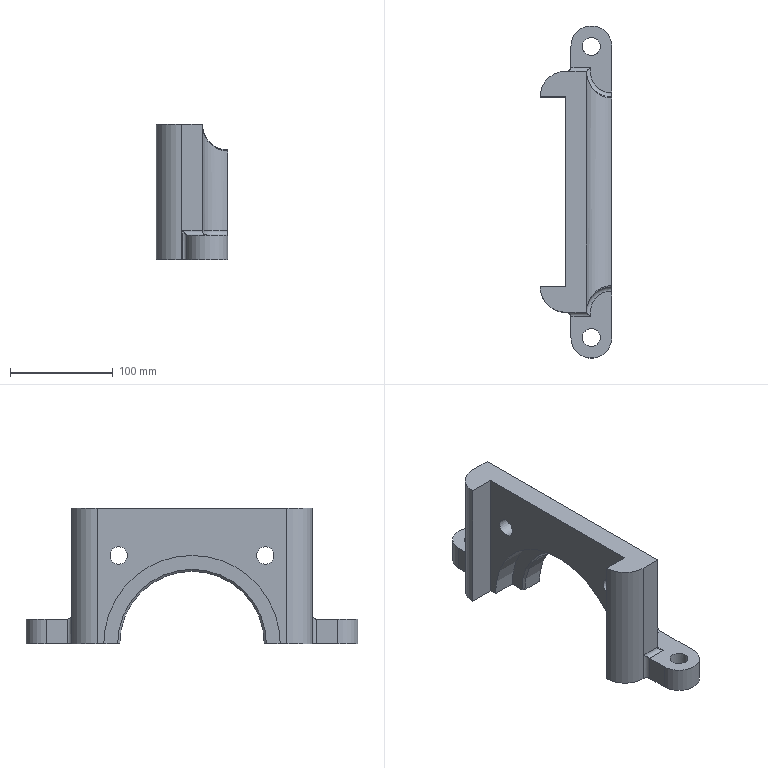Part | NX | features DATUM_CSYS 8, SKETCH 7, EXTRUDE 5, BLEND 4, CBORE_HOLE 2, HOLE PACKAGE 2, SIMPLE HOLE 2, CHAMFER 1, SWP104 1 | 1 solid | 40 faces | box 70 x 324 x 132 mm | volume 928360 mm3 | cylinder 19 | plane 16 | torus 2 | spline 2 | cone 1 | commonest cylinder face diameters 50 x5 8 x4 17 x2 17.5 x2 35 x2 40 x2
STEP:
#1=CARTESIAN_POINT('',(50.,71.5,103.5));
#2=VERTEX_POINT('',#1);
#3=CARTESIAN_POINT('',(50.,71.5,86.));
#4=DIRECTION('',(-1.,0.,0.));
#5=DIRECTION('',(0.,0.,1.));
#6=AXIS2_PLACEMENT_3D('',#3,#4,#5);
#7=CIRCLE('',#6,17.5);
#8=EDGE_CURVE('',#2,#2,#7,.T.);
#9=ORIENTED_EDGE('',*,*,#8,.T.);
#10=EDGE_LOOP('',(#9));
#11=FACE_BOUND('',#10,.T.);
#12=CARTESIAN_POINT('',(50.,-71.5,103.5));
#13=VERTEX_POINT('',#12);
#14=CARTESIAN_POINT('',(50.,-71.5,86.));
#15=DIRECTION('',(-1.,0.,0.));
#16=DIRECTION('',(0.,0.,1.));
#17=AXIS2_PLACEMENT_3D('',#14,#15,#16);
#18=CIRCLE('',#17,17.5);
#19=EDGE_CURVE('',#13,#13,#18,.T.);
#20=ORIENTED_EDGE('',*,*,#19,.T.);
#21=EDGE_LOOP('',(#20));
#22=FACE_BOUND('',#21,.T.);
#23=CARTESIAN_POINT('',(50.,92.5,28.));
#24=VERTEX_POINT('',#23);
#25=CARTESIAN_POINT('',(50.,92.5,106.));
#26=VERTEX_POINT('',#25);
#27=CARTESIAN_POINT('',(50.,92.5,142.8));
#28=DIRECTION('',(0.,0.,-1.));
#29=VECTOR('',#28,1000.);
#30=LINE('',#27,#29);
#31=EDGE_CURVE('',#24,#26,#30,.F.);
#32=ORIENTED_EDGE('',*,*,#31,.T.);
#33=CARTESIAN_POINT('',(50.,91.5,107.));
#34=VERTEX_POINT('',#33);
#35=CARTESIAN_POINT('',(50.,91.5,106.));
#36=DIRECTION('',(1.,0.,0.));
#37=DIRECTION('',(0.,0.,-1.));
#38=AXIS2_PLACEMENT_3D('',#35,#36,#37);
#39=CIRCLE('',#38,1.);
#40=EDGE_CURVE('',#26,#34,#39,.T.);
#41=ORIENTED_EDGE('',*,*,#40,.T.);
#42=CARTESIAN_POINT('',(50.,-91.5,107.));
#43=VERTEX_POINT('',#42);
#44=CARTESIAN_POINT('',(50.,-178.2,107.));
#45=DIRECTION('',(0.,1.,0.));
#46=VECTOR('',#45,1000.);
#47=LINE('',#44,#46);
#48=EDGE_CURVE('',#34,#43,#47,.F.);
#49=ORIENTED_EDGE('',*,*,#48,.T.);
#50=CARTESIAN_POINT('',(50.,-92.5,106.));
#51=VERTEX_POINT('',#50);
#52=CARTESIAN_POINT('',(50.,-91.5,106.));
#53=DIRECTION('',(1.,0.,0.));
#54=DIRECTION('',(0.,0.,-1.));
#55=AXIS2_PLACEMENT_3D('',#52,#53,#54);
#56=CIRCLE('',#55,1.);
#57=EDGE_CURVE('',#43,#51,#56,.T.);
#58=ORIENTED_EDGE('',*,*,#57,.T.);
#59=CARTESIAN_POINT('',(50.,-92.5,28.));
#60=VERTEX_POINT('',#59);
#61=CARTESIAN_POINT('',(50.,-92.5,142.8));
#62=DIRECTION('',(0.,0.,-1.));
#63=VECTOR('',#62,1000.);
#64=LINE('',#61,#63);
#65=EDGE_CURVE('',#60,#51,#64,.F.);
#66=ORIENTED_EDGE('',*,*,#65,.F.);
#67=CARTESIAN_POINT('',(50.,-96.5,24.));
#68=VERTEX_POINT('',#67);
#69=CARTESIAN_POINT('',(50.,-96.5,28.));
#70=DIRECTION('',(1.,0.,0.));
#71=DIRECTION('',(0.,0.,-1.));
#72=AXIS2_PLACEMENT_3D('',#69,#70,#71);
#73=CIRCLE('',#72,4.);
#74=EDGE_CURVE('',#60,#68,#73,.F.);
#75=ORIENTED_EDGE('',*,*,#74,.T.);
#76=CARTESIAN_POINT('',(50.,-142.,24.));
#77=VERTEX_POINT('',#76);
#78=CARTESIAN_POINT('',(50.,-117.5,24.));
#79=DIRECTION('',(0.,-1.,0.));
#80=VECTOR('',#79,1000.);
#81=LINE('',#78,#80);
#82=EDGE_CURVE('',#68,#77,#81,.T.);
#83=ORIENTED_EDGE('',*,*,#82,.T.);
#84=CARTESIAN_POINT('',(50.,-142.,0.));
#85=VERTEX_POINT('',#84);
#86=CARTESIAN_POINT('',(50.,-142.,0.));
#87=DIRECTION('',(0.,0.,-1.));
#88=VECTOR('',#87,1000.);
#89=LINE('',#86,#88);
#90=EDGE_CURVE('',#77,#85,#89,.T.);
#91=ORIENTED_EDGE('',*,*,#90,.T.);
#92=CARTESIAN_POINT('',(50.,-70.5,0.));
#93=VERTEX_POINT('',#92);
#94=CARTESIAN_POINT('',(50.,-162.,0.));
#95=DIRECTION('',(0.,1.,0.));
#96=VECTOR('',#95,1000.);
#97=LINE('',#94,#96);
#98=EDGE_CURVE('',#85,#93,#97,.T.);
#99=ORIENTED_EDGE('',*,*,#98,.T.);
#100=CARTESIAN_POINT('',(50.,70.5,0.));
#101=VERTEX_POINT('',#100);
#102=CARTESIAN_POINT('',(50.,0.,0.));
#103=DIRECTION('',(1.,0.,0.));
#104=DIRECTION('',(0.,0.,-1.));
#105=AXIS2_PLACEMENT_3D('',#102,#103,#104);
#106=CIRCLE('',#105,70.5);
#107=EDGE_CURVE('',#101,#93,#106,.T.);
#108=ORIENTED_EDGE('',*,*,#107,.F.);
#109=CARTESIAN_POINT('',(50.,142.,0.));
#110=VERTEX_POINT('',#109);
#111=CARTESIAN_POINT('',(50.,-162.,0.));
#112=DIRECTION('',(0.,1.,0.));
#113=VECTOR('',#112,1000.);
#114=LINE('',#111,#113);
#115=EDGE_CURVE('',#101,#110,#114,.T.);
#116=ORIENTED_EDGE('',*,*,#115,.T.);
#117=CARTESIAN_POINT('',(50.,142.,24.));
#118=VERTEX_POINT('',#117);
#119=CARTESIAN_POINT('',(50.,142.,24.));
#120=DIRECTION('',(0.,0.,1.));
#121=VECTOR('',#120,1000.);
#122=LINE('',#119,#121);
#123=EDGE_CURVE('',#110,#118,#122,.T.);
#124=ORIENTED_EDGE('',*,*,#123,.T.);
#125=CARTESIAN_POINT('',(50.,96.5,24.));
#126=VERTEX_POINT('',#125);
#127=CARTESIAN_POINT('',(50.,162.,24.));
#128=DIRECTION('',(0.,-1.,0.));
#129=VECTOR('',#128,1000.);
#130=LINE('',#127,#129);
#131=EDGE_CURVE('',#118,#126,#130,.T.);
#132=ORIENTED_EDGE('',*,*,#131,.T.);
#133=CARTESIAN_POINT('',(50.,96.5,28.));
#134=DIRECTION('',(1.,0.,0.));
#135=DIRECTION('',(0.,0.,-1.));
#136=AXIS2_PLACEMENT_3D('',#133,#134,#135);
#137=CIRCLE('',#136,4.);
#138=EDGE_CURVE('',#126,#24,#137,.F.);
#139=ORIENTED_EDGE('',*,*,#138,.T.);
#140=EDGE_LOOP('',(#32,#41,#49,#58,#66,#75,#83,#91,#99,#108,#116,#124,#132,#139));
#141=FACE_BOUND('',#140,.T.);
#142=CARTESIAN_POINT('',(50.,0.,0.));
#143=DIRECTION('',(1.,0.,0.));
#144=DIRECTION('',(0.,0.,-1.));
#145=AXIS2_PLACEMENT_3D('',#142,#143,#144);
#146=PLANE('',#145);
#147=ADVANCED_FACE('',(#11,#22,#141),#146,.T.);
#148=CARTESIAN_POINT('',(25.,117.5,28.));
#149=VERTEX_POINT('',#148);
#150=CARTESIAN_POINT('',(6.,117.5,28.));
#151=VERTEX_POINT('',#150);
#152=CARTESIAN_POINT('',(10.,117.5,28.));
#153=DIRECTION('',(-1.,0.,0.));
#154=VECTOR('',#153,1000.);
#155=LINE('',#152,#154);
#156=EDGE_CURVE('',#149,#151,#155,.T.);
#157=ORIENTED_EDGE('',*,*,#156,.T.);
#158=CARTESIAN_POINT('',(6.,117.5,0.));
#159=VERTEX_POINT('',#158);
#160=CARTESIAN_POINT('',(6.,117.5,0.));
#161=DIRECTION('',(0.,0.,-1.));
#162=VECTOR('',#161,1000.);
#163=LINE('',#160,#162);
#164=EDGE_CURVE('',#151,#159,#163,.T.);
#165=ORIENTED_EDGE('',*,*,#164,.T.);
#166=CARTESIAN_POINT('',(5.,117.5,0.));
#167=VERTEX_POINT('',#166);
#168=CARTESIAN_POINT('',(10.,117.5,0.));
#169=DIRECTION('',(-1.,0.,0.));
#170=VECTOR('',#169,1000.);
#171=LINE('',#168,#170);
#172=EDGE_CURVE('',#167,#159,#171,.F.);
#173=ORIENTED_EDGE('',*,*,#172,.F.);
#174=CARTESIAN_POINT('',(5.,117.5,132.));
#175=VERTEX_POINT('',#174);
#176=CARTESIAN_POINT('',(5.,117.5,24.));
#177=DIRECTION('',(0.,0.,1.));
#178=VECTOR('',#177,1000.);
#179=LINE('',#176,#178);
#180=EDGE_CURVE('',#167,#175,#179,.T.);
#181=ORIENTED_EDGE('',*,*,#180,.T.);
#182=CARTESIAN_POINT('',(25.,117.5,132.));
#183=VERTEX_POINT('',#182);
#184=CARTESIAN_POINT('',(50.,117.5,132.));
#185=DIRECTION('',(-1.,0.,0.));
#186=VECTOR('',#185,1000.);
#187=LINE('',#184,#186);
#188=EDGE_CURVE('',#183,#175,#187,.T.);
#189=ORIENTED_EDGE('',*,*,#188,.F.);
#190=CARTESIAN_POINT('',(25.,117.5,142.8));
#191=DIRECTION('',(0.,0.,-1.));
#192=VECTOR('',#191,1000.);
#193=LINE('',#190,#192);
#194=EDGE_CURVE('',#149,#183,#193,.F.);
#195=ORIENTED_EDGE('',*,*,#194,.F.);
#196=EDGE_LOOP('',(#157,#165,#173,#181,#189,#195));
#197=FACE_BOUND('',#196,.T.);
#198=CARTESIAN_POINT('',(50.,117.5,24.));
#199=DIRECTION('',(0.,-1.,0.));
#200=DIRECTION('',(0.,0.,-1.));
#201=AXIS2_PLACEMENT_3D('',#198,#199,#200);
#202=PLANE('',#201);
#203=ADVANCED_FACE('',(#197),#202,.F.);
#204=ORIENTED_EDGE('',*,*,#48,.F.);
#205=CARTESIAN_POINT('',(50.,117.5,132.));
#206=DIRECTION('',(0.,-0.6931,0.7208));
#207=DIRECTION('',(0.,0.7208,0.6931));
#208=AXIS2_PLACEMENT_3D('',#205,#206,#207);
#209=ELLIPSE('',#208,36.069,25.);
#210=EDGE_CURVE('',#34,#183,#209,.F.);
#211=ORIENTED_EDGE('',*,*,#210,.T.);
#212=CARTESIAN_POINT('',(25.,-117.5,132.));
#213=VERTEX_POINT('',#212);
#214=CARTESIAN_POINT('',(25.,-178.2,132.));
#215=DIRECTION('',(0.,1.,0.));
#216=VECTOR('',#215,1000.);
#217=LINE('',#214,#216);
#218=EDGE_CURVE('',#183,#213,#217,.F.);
#219=ORIENTED_EDGE('',*,*,#218,.T.);
#220=CARTESIAN_POINT('',(50.,-117.5,132.));
#221=DIRECTION('',(0.,0.6931,0.7208));
#222=DIRECTION('',(0.,0.7208,-0.6931));
#223=AXIS2_PLACEMENT_3D('',#220,#221,#222);
#224=ELLIPSE('',#223,36.069,25.);
#225=EDGE_CURVE('',#213,#43,#224,.F.);
#226=ORIENTED_EDGE('',*,*,#225,.T.);
#227=EDGE_LOOP('',(#204,#211,#219,#226));
#228=FACE_BOUND('',#227,.T.);
#229=CARTESIAN_POINT('',(50.,-178.2,132.));
#230=DIRECTION('',(0.,1.,0.));
#231=DIRECTION('',(0.,0.,1.));
#232=AXIS2_PLACEMENT_3D('',#229,#230,#231);
#233=CYLINDRICAL_SURFACE('',#232,25.);
#234=ADVANCED_FACE('',(#228),#233,.F.);
#235=CARTESIAN_POINT('',(38.75,142.,0.));
#236=VERTEX_POINT('',#235);
#237=CARTESIAN_POINT('',(30.,142.,0.));
#238=DIRECTION('',(0.,0.,1.));
#239=DIRECTION('',(1.,0.,0.));
#240=AXIS2_PLACEMENT_3D('',#237,#238,#239);
#241=CIRCLE('',#240,8.75);
#242=EDGE_CURVE('',#236,#236,#241,.T.);
#243=ORIENTED_EDGE('',*,*,#242,.T.);
#244=EDGE_LOOP('',(#243));
#245=FACE_BOUND('',#244,.T.);
#246=CARTESIAN_POINT('',(30.,70.5,0.));
#247=VERTEX_POINT('',#246);
#248=CARTESIAN_POINT('',(50.,70.5,0.));
#249=DIRECTION('',(1.,0.,0.));
#250=VECTOR('',#249,1000.);
#251=LINE('',#248,#250);
#252=EDGE_CURVE('',#101,#247,#251,.F.);
#253=ORIENTED_EDGE('',*,*,#252,.T.);
#254=CARTESIAN_POINT('',(28.,72.5,0.));
#255=VERTEX_POINT('',#254);
#256=CARTESIAN_POINT('',(100.5,0.,0.));
#257=DIRECTION('',(-0.7071,0.7071,0.));
#258=VECTOR('',#257,1000.);
#259=LINE('',#256,#258);
#260=EDGE_CURVE('',#247,#255,#259,.T.);
#261=ORIENTED_EDGE('',*,*,#260,.T.);
#262=CARTESIAN_POINT('',(28.,86.,0.));
#263=VERTEX_POINT('',#262);
#264=CARTESIAN_POINT('',(28.,-162.,0.));
#265=DIRECTION('',(0.,1.,0.));
#266=VECTOR('',#265,1000.);
#267=LINE('',#264,#266);
#268=EDGE_CURVE('',#255,#263,#267,.T.);
#269=ORIENTED_EDGE('',*,*,#268,.T.);
#270=CARTESIAN_POINT('',(5.,86.,0.));
#271=VERTEX_POINT('',#270);
#272=CARTESIAN_POINT('',(50.,86.,0.));
#273=DIRECTION('',(1.,0.,0.));
#274=VECTOR('',#273,1000.);
#275=LINE('',#272,#274);
#276=EDGE_CURVE('',#263,#271,#275,.F.);
#277=ORIENTED_EDGE('',*,*,#276,.T.);
#278=CARTESIAN_POINT('',(5.,92.5,0.));
#279=VERTEX_POINT('',#278);
#280=CARTESIAN_POINT('',(5.,92.5,0.));
#281=DIRECTION('',(0.,-1.,0.));
#282=VECTOR('',#281,1000.);
#283=LINE('',#280,#282);
#284=EDGE_CURVE('',#279,#271,#283,.T.);
#285=ORIENTED_EDGE('',*,*,#284,.F.);
#286=CARTESIAN_POINT('',(-20.,92.5,0.));
#287=VERTEX_POINT('',#286);
#288=CARTESIAN_POINT('',(-20.,92.5,0.));
#289=DIRECTION('',(1.,0.,0.));
#290=VECTOR('',#289,1000.);
#291=LINE('',#288,#290);
#292=EDGE_CURVE('',#287,#279,#291,.T.);
#293=ORIENTED_EDGE('',*,*,#292,.F.);
#294=CARTESIAN_POINT('',(5.,92.5,0.));
#295=DIRECTION('',(0.,0.,1.));
#296=DIRECTION('',(1.,0.,0.));
#297=AXIS2_PLACEMENT_3D('',#294,#295,#296);
#298=CIRCLE('',#297,25.);
#299=EDGE_CURVE('',#287,#167,#298,.F.);
#300=ORIENTED_EDGE('',*,*,#299,.T.);
#301=ORIENTED_EDGE('',*,*,#172,.T.);
#302=CARTESIAN_POINT('',(10.,121.5,0.));
#303=VERTEX_POINT('',#302);
#304=CARTESIAN_POINT('',(6.,121.5,0.));
#305=DIRECTION('',(0.,0.,1.));
#306=DIRECTION('',(1.,0.,0.));
#307=AXIS2_PLACEMENT_3D('',#304,#305,#306);
#308=CIRCLE('',#307,4.);
#309=EDGE_CURVE('',#159,#303,#308,.T.);
#310=ORIENTED_EDGE('',*,*,#309,.T.);
#311=CARTESIAN_POINT('',(10.,142.,0.));
#312=VERTEX_POINT('',#311);
#313=CARTESIAN_POINT('',(10.,162.,0.));
#314=DIRECTION('',(0.,-1.,0.));
#315=VECTOR('',#314,1000.);
#316=LINE('',#313,#315);
#317=EDGE_CURVE('',#312,#303,#316,.T.);
#318=ORIENTED_EDGE('',*,*,#317,.F.);
#319=CARTESIAN_POINT('',(30.,142.,0.));
#320=DIRECTION('',(0.,0.,1.));
#321=DIRECTION('',(1.,0.,0.));
#322=AXIS2_PLACEMENT_3D('',#319,#320,#321);
#323=CIRCLE('',#322,20.);
#324=EDGE_CURVE('',#312,#110,#323,.F.);
#325=ORIENTED_EDGE('',*,*,#324,.T.);
#326=ORIENTED_EDGE('',*,*,#115,.F.);
#327=EDGE_LOOP('',(#253,#261,#269,#277,#285,#293,#300,#301,#310,#318,#325,#326));
#328=FACE_BOUND('',#327,.T.);
#329=CARTESIAN_POINT('',(50.,-162.,0.));
#330=DIRECTION('',(0.,0.,1.));
#331=DIRECTION('',(1.,0.,0.));
#332=AXIS2_PLACEMENT_3D('',#329,#330,#331);
#333=PLANE('',#332);
#334=ADVANCED_FACE('',(#245,#328),#333,.F.);
#335=CARTESIAN_POINT('',(38.75,-142.,0.));
#336=VERTEX_POINT('',#335);
#337=CARTESIAN_POINT('',(30.,-142.,0.));
#338=DIRECTION('',(0.,0.,1.));
#339=DIRECTION('',(1.,0.,0.));
#340=AXIS2_PLACEMENT_3D('',#337,#338,#339);
#341=CIRCLE('',#340,8.75);
#342=EDGE_CURVE('',#336,#336,#341,.T.);
#343=ORIENTED_EDGE('',*,*,#342,.T.);
#344=EDGE_LOOP('',(#343));
#345=FACE_BOUND('',#344,.T.);
#346=CARTESIAN_POINT('',(28.,-86.,0.));
#347=VERTEX_POINT('',#346);
#348=CARTESIAN_POINT('',(28.,-72.5,0.));
#349=VERTEX_POINT('',#348);
#350=CARTESIAN_POINT('',(28.,-162.,0.));
#351=DIRECTION('',(0.,1.,0.));
#352=VECTOR('',#351,1000.);
#353=LINE('',#350,#352);
#354=EDGE_CURVE('',#347,#349,#353,.T.);
#355=ORIENTED_EDGE('',*,*,#354,.T.);
#356=CARTESIAN_POINT('',(30.,-70.5,0.));
#357=VERTEX_POINT('',#356);
#358=CARTESIAN_POINT('',(100.5,0.,0.));
#359=DIRECTION('',(0.7071,0.7071,0.));
#360=VECTOR('',#359,1000.);
#361=LINE('',#358,#360);
#362=EDGE_CURVE('',#349,#357,#361,.T.);
#363=ORIENTED_EDGE('',*,*,#362,.T.);
#364=CARTESIAN_POINT('',(50.,-70.5,0.));
#365=DIRECTION('',(1.,0.,0.));
#366=VECTOR('',#365,1000.);
#367=LINE('',#364,#366);
#368=EDGE_CURVE('',#357,#93,#367,.T.);
#369=ORIENTED_EDGE('',*,*,#368,.T.);
#370=ORIENTED_EDGE('',*,*,#98,.F.);
#371=CARTESIAN_POINT('',(10.,-142.,0.));
#372=VERTEX_POINT('',#371);
#373=CARTESIAN_POINT('',(30.,-142.,0.));
#374=DIRECTION('',(0.,0.,1.));
#375=DIRECTION('',(1.,0.,0.));
#376=AXIS2_PLACEMENT_3D('',#373,#374,#375);
#377=CIRCLE('',#376,20.);
#378=EDGE_CURVE('',#85,#372,#377,.F.);
#379=ORIENTED_EDGE('',*,*,#378,.T.);
#380=CARTESIAN_POINT('',(10.,-121.5,0.));
#381=VERTEX_POINT('',#380);
#382=CARTESIAN_POINT('',(10.,-162.,0.));
#383=DIRECTION('',(0.,1.,0.));
#384=VECTOR('',#383,1000.);
#385=LINE('',#382,#384);
#386=EDGE_CURVE('',#372,#381,#385,.T.);
#387=ORIENTED_EDGE('',*,*,#386,.T.);
#388=CARTESIAN_POINT('',(6.,-117.5,0.));
#389=VERTEX_POINT('',#388);
#390=CARTESIAN_POINT('',(6.,-121.5,0.));
#391=DIRECTION('',(0.,0.,1.));
#392=DIRECTION('',(1.,0.,0.));
#393=AXIS2_PLACEMENT_3D('',#390,#391,#392);
#394=CIRCLE('',#393,4.);
#395=EDGE_CURVE('',#381,#389,#394,.T.);
#396=ORIENTED_EDGE('',*,*,#395,.T.);
#397=CARTESIAN_POINT('',(5.,-117.5,0.));
#398=VERTEX_POINT('',#397);
#399=CARTESIAN_POINT('',(10.,-117.5,0.));
#400=DIRECTION('',(-1.,0.,0.));
#401=VECTOR('',#400,1000.);
#402=LINE('',#399,#401);
#403=EDGE_CURVE('',#389,#398,#402,.T.);
#404=ORIENTED_EDGE('',*,*,#403,.T.);
#405=CARTESIAN_POINT('',(-20.,-92.5,0.));
#406=VERTEX_POINT('',#405);
#407=CARTESIAN_POINT('',(5.,-92.5,0.));
#408=DIRECTION('',(0.,0.,1.));
#409=DIRECTION('',(1.,0.,0.));
#410=AXIS2_PLACEMENT_3D('',#407,#408,#409);
#411=CIRCLE('',#410,25.);
#412=EDGE_CURVE('',#398,#406,#411,.F.);
#413=ORIENTED_EDGE('',*,*,#412,.T.);
#414=CARTESIAN_POINT('',(5.,-92.5,0.));
#415=VERTEX_POINT('',#414);
#416=CARTESIAN_POINT('',(5.,-92.5,0.));
#417=DIRECTION('',(-1.,0.,0.));
#418=VECTOR('',#417,1000.);
#419=LINE('',#416,#418);
#420=EDGE_CURVE('',#415,#406,#419,.T.);
#421=ORIENTED_EDGE('',*,*,#420,.F.);
#422=CARTESIAN_POINT('',(5.,-86.,0.));
#423=VERTEX_POINT('',#422);
#424=CARTESIAN_POINT('',(5.,92.5,0.));
#425=DIRECTION('',(0.,-1.,0.));
#426=VECTOR('',#425,1000.);
#427=LINE('',#424,#426);
#428=EDGE_CURVE('',#423,#415,#427,.T.);
#429=ORIENTED_EDGE('',*,*,#428,.F.);
#430=CARTESIAN_POINT('',(50.,-86.,0.));
#431=DIRECTION('',(1.,0.,0.));
#432=VECTOR('',#431,1000.);
#433=LINE('',#430,#432);
#434=EDGE_CURVE('',#423,#347,#433,.T.);
#435=ORIENTED_EDGE('',*,*,#434,.T.);
#436=EDGE_LOOP('',(#355,#363,#369,#370,#379,#387,#396,#404,#413,#421,#429,#435));
#437=FACE_BOUND('',#436,.T.);
#438=CARTESIAN_POINT('',(50.,-162.,0.));
#439=DIRECTION('',(0.,0.,1.));
#440=DIRECTION('',(1.,0.,0.));
#441=AXIS2_PLACEMENT_3D('',#438,#439,#440);
#442=PLANE('',#441);
#443=ADVANCED_FACE('',(#345,#437),#442,.F.);
#444=CARTESIAN_POINT('',(5.,-92.5,132.));
#445=VERTEX_POINT('',#444);
#446=CARTESIAN_POINT('',(-20.,-92.5,132.));
#447=VERTEX_POINT('',#446);
#448=CARTESIAN_POINT('',(50.,-92.5,132.));
#449=DIRECTION('',(-1.,0.,0.));
#450=VECTOR('',#449,1000.);
#451=LINE('',#448,#450);
#452=EDGE_CURVE('',#445,#447,#451,.T.);
#453=ORIENTED_EDGE('',*,*,#452,.T.);
#454=CARTESIAN_POINT('',(5.,-117.5,132.));
#455=VERTEX_POINT('',#454);
#456=CARTESIAN_POINT('',(5.,-92.5,132.));
#457=DIRECTION('',(0.,0.,-1.));
#458=DIRECTION('',(0.,1.,0.));
#459=AXIS2_PLACEMENT_3D('',#456,#457,#458);
#460=CIRCLE('',#459,25.);
#461=EDGE_CURVE('',#447,#455,#460,.F.);
#462=ORIENTED_EDGE('',*,*,#461,.T.);
#463=CARTESIAN_POINT('',(50.,-117.5,132.));
#464=DIRECTION('',(-1.,0.,0.));
#465=VECTOR('',#464,1000.);
#466=LINE('',#463,#465);
#467=EDGE_CURVE('',#213,#455,#466,.T.);
#468=ORIENTED_EDGE('',*,*,#467,.F.);
#469=ORIENTED_EDGE('',*,*,#218,.F.);
#470=ORIENTED_EDGE('',*,*,#188,.T.);
#471=CARTESIAN_POINT('',(-20.,92.5,132.));
#472=VERTEX_POINT('',#471);
#473=CARTESIAN_POINT('',(5.,92.5,132.));
#474=DIRECTION('',(0.,0.,-1.));
#475=DIRECTION('',(0.,1.,0.));
#476=AXIS2_PLACEMENT_3D('',#473,#474,#475);
#477=CIRCLE('',#476,25.);
#478=EDGE_CURVE('',#175,#472,#477,.F.);
#479=ORIENTED_EDGE('',*,*,#478,.T.);
#480=CARTESIAN_POINT('',(5.,92.5,132.));
#481=VERTEX_POINT('',#480);
#482=CARTESIAN_POINT('',(50.,92.5,132.));
#483=DIRECTION('',(1.,0.,0.));
#484=VECTOR('',#483,1000.);
#485=LINE('',#482,#484);
#486=EDGE_CURVE('',#472,#481,#485,.T.);
#487=ORIENTED_EDGE('',*,*,#486,.T.);
#488=CARTESIAN_POINT('',(5.,117.5,132.));
#489=DIRECTION('',(0.,-1.,0.));
#490=VECTOR('',#489,1000.);
#491=LINE('',#488,#490);
#492=EDGE_CURVE('',#481,#445,#491,.T.);
#493=ORIENTED_EDGE('',*,*,#492,.T.);
#494=EDGE_LOOP('',(#453,#462,#468,#469,#470,#479,#487,#493));
#495=FACE_BOUND('',#494,.T.);
#496=CARTESIAN_POINT('',(50.,117.5,132.));
#497=DIRECTION('',(0.,0.,-1.));
#498=DIRECTION('',(0.,1.,0.));
#499=AXIS2_PLACEMENT_3D('',#496,#497,#498);
#500=PLANE('',#499);
#501=ADVANCED_FACE('',(#495),#500,.F.);
#502=CARTESIAN_POINT('',(30.,150.75,24.));
#503=VERTEX_POINT('',#502);
#504=CARTESIAN_POINT('',(30.,142.,24.));
#505=DIRECTION('',(0.,0.,-1.));
#506=DIRECTION('',(0.,1.,0.));
#507=AXIS2_PLACEMENT_3D('',#504,#505,#506);
#508=CIRCLE('',#507,8.75);
#509=EDGE_CURVE('',#503,#503,#508,.T.);
#510=ORIENTED_EDGE('',*,*,#509,.T.);
#511=EDGE_LOOP('',(#510));
#512=FACE_BOUND('',#511,.T.);
#513=CARTESIAN_POINT('',(10.,121.5,24.));
#514=VERTEX_POINT('',#513);
#515=CARTESIAN_POINT('',(10.,142.,24.));
#516=VERTEX_POINT('',#515);
#517=CARTESIAN_POINT('',(10.,162.,24.));
#518=DIRECTION('',(0.,1.,0.));
#519=VECTOR('',#518,1000.);
#520=LINE('',#517,#519);
#521=EDGE_CURVE('',#514,#516,#520,.T.);
#522=ORIENTED_EDGE('',*,*,#521,.F.);
#523=CARTESIAN_POINT('',(29.384,121.5,24.));
#524=VERTEX_POINT('',#523);
#525=CARTESIAN_POINT('',(25.,121.5,24.));
#526=DIRECTION('',(-1.,0.,0.));
#527=VECTOR('',#526,1000.);
#528=LINE('',#525,#527);
#529=EDGE_CURVE('',#514,#524,#528,.F.);
#530=ORIENTED_EDGE('',*,*,#529,.T.);
#531=CARTESIAN_POINT('',(50.,117.5,24.));
#532=DIRECTION('',(0.,0.,-1.));
#533=DIRECTION('',(0.,1.,0.));
#534=AXIS2_PLACEMENT_3D('',#531,#532,#533);
#535=CIRCLE('',#534,21.);
#536=EDGE_CURVE('',#524,#126,#535,.F.);
#537=ORIENTED_EDGE('',*,*,#536,.T.);
#538=ORIENTED_EDGE('',*,*,#131,.F.);
#539=CARTESIAN_POINT('',(30.,142.,24.));
#540=DIRECTION('',(0.,0.,-1.));
#541=DIRECTION('',(0.,1.,0.));
#542=AXIS2_PLACEMENT_3D('',#539,#540,#541);
#543=CIRCLE('',#542,20.);
#544=EDGE_CURVE('',#118,#516,#543,.F.);
#545=ORIENTED_EDGE('',*,*,#544,.T.);
#546=EDGE_LOOP('',(#522,#530,#537,#538,#545));
#547=FACE_BOUND('',#546,.T.);
#548=CARTESIAN_POINT('',(50.,162.,24.));
#549=DIRECTION('',(0.,0.,-1.));
#550=DIRECTION('',(0.,1.,0.));
#551=AXIS2_PLACEMENT_3D('',#548,#549,#550);
#552=PLANE('',#551);
#553=ADVANCED_FACE('',(#512,#547),#552,.F.);
#554=ORIENTED_EDGE('',*,*,#403,.F.);
#555=CARTESIAN_POINT('',(6.,-117.5,28.));
#556=VERTEX_POINT('',#555);
#557=CARTESIAN_POINT('',(6.,-117.5,132.));
#558=DIRECTION('',(0.,0.,-1.));
#559=VECTOR('',#558,1000.);
#560=LINE('',#557,#559);
#561=EDGE_CURVE('',#389,#556,#560,.F.);
#562=ORIENTED_EDGE('',*,*,#561,.T.);
#563=CARTESIAN_POINT('',(25.,-117.5,28.));
#564=VERTEX_POINT('',#563);
#565=CARTESIAN_POINT('',(25.,-117.5,28.));
#566=DIRECTION('',(-1.,0.,0.));
#567=VECTOR('',#566,1000.);
#568=LINE('',#565,#567);
#569=EDGE_CURVE('',#556,#564,#568,.F.);
#570=ORIENTED_EDGE('',*,*,#569,.T.);
#571=CARTESIAN_POINT('',(25.,-117.5,142.8));
#572=DIRECTION('',(0.,0.,-1.));
#573=VECTOR('',#572,1000.);
#574=LINE('',#571,#573);
#575=EDGE_CURVE('',#564,#213,#574,.F.);
#576=ORIENTED_EDGE('',*,*,#575,.T.);
#577=ORIENTED_EDGE('',*,*,#467,.T.);
#578=CARTESIAN_POINT('',(5.,-117.5,132.));
#579=DIRECTION('',(0.,0.,-1.));
#580=VECTOR('',#579,1000.);
#581=LINE('',#578,#580);
#582=EDGE_CURVE('',#455,#398,#581,.T.);
#583=ORIENTED_EDGE('',*,*,#582,.T.);
#584=EDGE_LOOP('',(#554,#562,#570,#576,#577,#583));
#585=FACE_BOUND('',#584,.T.);
#586=CARTESIAN_POINT('',(50.,-117.5,132.));
#587=DIRECTION('',(0.,1.,0.));
#588=DIRECTION('',(0.,0.,1.));
#589=AXIS2_PLACEMENT_3D('',#586,#587,#588);
#590=PLANE('',#589);
#591=ADVANCED_FACE('',(#585),#590,.F.);
#592=CARTESIAN_POINT('',(30.,-133.25,24.));
#593=VERTEX_POINT('',#592);
#594=CARTESIAN_POINT('',(30.,-142.,24.));
#595=DIRECTION('',(0.,0.,-1.));
#596=DIRECTION('',(0.,1.,0.));
#597=AXIS2_PLACEMENT_3D('',#594,#595,#596);
#598=CIRCLE('',#597,8.75);
#599=EDGE_CURVE('',#593,#593,#598,.T.);
#600=ORIENTED_EDGE('',*,*,#599,.T.);
#601=EDGE_LOOP('',(#600));
#602=FACE_BOUND('',#601,.T.);
#603=CARTESIAN_POINT('',(29.384,-121.5,24.));
#604=VERTEX_POINT('',#603);
#605=CARTESIAN_POINT('',(50.,-117.5,24.));
#606=DIRECTION('',(0.,0.,-1.));
#607=DIRECTION('',(0.,1.,0.));
#608=AXIS2_PLACEMENT_3D('',#605,#606,#607);
#609=CIRCLE('',#608,21.);
#610=EDGE_CURVE('',#68,#604,#609,.F.);
#611=ORIENTED_EDGE('',*,*,#610,.T.);
#612=CARTESIAN_POINT('',(10.,-121.5,24.));
#613=VERTEX_POINT('',#612);
#614=CARTESIAN_POINT('',(10.,-121.5,24.));
#615=DIRECTION('',(-1.,0.,0.));
#616=VECTOR('',#615,1000.);
#617=LINE('',#614,#616);
#618=EDGE_CURVE('',#604,#613,#617,.T.);
#619=ORIENTED_EDGE('',*,*,#618,.T.);
#620=CARTESIAN_POINT('',(10.,-142.,24.));
#621=VERTEX_POINT('',#620);
#622=CARTESIAN_POINT('',(10.,-162.,24.));
#623=DIRECTION('',(0.,-1.,0.));
#624=VECTOR('',#623,1000.);
#625=LINE('',#622,#624);
#626=EDGE_CURVE('',#613,#621,#625,.T.);
#627=ORIENTED_EDGE('',*,*,#626,.T.);
#628=CARTESIAN_POINT('',(30.,-142.,24.));
#629=DIRECTION('',(0.,0.,-1.));
#630=DIRECTION('',(0.,1.,0.));
#631=AXIS2_PLACEMENT_3D('',#628,#629,#630);
#632=CIRCLE('',#631,20.);
#633=EDGE_CURVE('',#621,#77,#632,.F.);
#634=ORIENTED_EDGE('',*,*,#633,.T.);
#635=ORIENTED_EDGE('',*,*,#82,.F.);
#636=EDGE_LOOP('',(#611,#619,#627,#634,#635));
#637=FACE_BOUND('',#636,.T.);
#638=CARTESIAN_POINT('',(50.,-117.5,24.));
#639=DIRECTION('',(0.,0.,-1.));
#640=DIRECTION('',(0.,1.,0.));
#641=AXIS2_PLACEMENT_3D('',#638,#639,#640);
#642=PLANE('',#641);
#643=ADVANCED_FACE('',(#602,#637),#642,.F.);
#644=ORIENTED_EDGE('',*,*,#626,.F.);
#645=CARTESIAN_POINT('',(10.,-121.5,145.2));
#646=DIRECTION('',(0.,0.,-1.));
#647=VECTOR('',#646,1000.);
#648=LINE('',#645,#647);
#649=EDGE_CURVE('',#613,#381,#648,.T.);
#650=ORIENTED_EDGE('',*,*,#649,.T.);
#651=ORIENTED_EDGE('',*,*,#386,.F.);
#652=CARTESIAN_POINT('',(10.,-142.,24.));
#653=DIRECTION('',(0.,0.,-1.));
#654=VECTOR('',#653,1000.);
#655=LINE('',#652,#654);
#656=EDGE_CURVE('',#372,#621,#655,.F.);
#657=ORIENTED_EDGE('',*,*,#656,.T.);
#658=EDGE_LOOP('',(#644,#650,#651,#657));
#659=FACE_BOUND('',#658,.T.);
#660=CARTESIAN_POINT('',(10.,-162.,145.2));
#661=DIRECTION('',(-1.,0.,0.));
#662=DIRECTION('',(0.,-1.,0.));
#663=AXIS2_PLACEMENT_3D('',#660,#661,#662);
#664=PLANE('',#663);
#665=ADVANCED_FACE('',(#659),#664,.T.);
#666=ORIENTED_EDGE('',*,*,#317,.T.);
#667=CARTESIAN_POINT('',(10.,121.5,24.));
#668=DIRECTION('',(0.,0.,-1.));
#669=VECTOR('',#668,1000.);
#670=LINE('',#667,#669);
#671=EDGE_CURVE('',#303,#514,#670,.F.);
#672=ORIENTED_EDGE('',*,*,#671,.T.);
#673=ORIENTED_EDGE('',*,*,#521,.T.);
#674=CARTESIAN_POINT('',(10.,142.,145.2));
#675=DIRECTION('',(0.,0.,-1.));
#676=VECTOR('',#675,1000.);
#677=LINE('',#674,#676);
#678=EDGE_CURVE('',#516,#312,#677,.T.);
#679=ORIENTED_EDGE('',*,*,#678,.T.);
#680=EDGE_LOOP('',(#666,#672,#673,#679));
#681=FACE_BOUND('',#680,.T.);
#682=CARTESIAN_POINT('',(10.,162.,145.2));
#683=DIRECTION('',(1.,0.,0.));
#684=DIRECTION('',(0.,1.,0.));
#685=AXIS2_PLACEMENT_3D('',#682,#683,#684);
#686=PLANE('',#685);
#687=ADVANCED_FACE('',(#681),#686,.F.);
#688=ORIENTED_EDGE('',*,*,#90,.F.);
#689=ORIENTED_EDGE('',*,*,#633,.F.);
#690=ORIENTED_EDGE('',*,*,#656,.F.);
#691=ORIENTED_EDGE('',*,*,#378,.F.);
#692=EDGE_LOOP('',(#688,#689,#690,#691));
#693=FACE_BOUND('',#692,.T.);
#694=CARTESIAN_POINT('',(30.,-142.,0.));
#695=DIRECTION('',(0.,0.,1.));
#696=DIRECTION('',(1.,0.,0.));
#697=AXIS2_PLACEMENT_3D('',#694,#695,#696);
#698=CYLINDRICAL_SURFACE('',#697,20.);
#699=ADVANCED_FACE('',(#693),#698,.T.);
#700=ORIENTED_EDGE('',*,*,#324,.F.);
#701=ORIENTED_EDGE('',*,*,#678,.F.);
#702=ORIENTED_EDGE('',*,*,#544,.F.);
#703=ORIENTED_EDGE('',*,*,#123,.F.);
#704=EDGE_LOOP('',(#700,#701,#702,#703));
#705=FACE_BOUND('',#704,.T.);
#706=CARTESIAN_POINT('',(30.,142.,0.));
#707=DIRECTION('',(0.,0.,-1.));
#708=DIRECTION('',(-1.,0.,0.));
#709=AXIS2_PLACEMENT_3D('',#706,#707,#708);
#710=CYLINDRICAL_SURFACE('',#709,20.);
#711=ADVANCED_FACE('',(#705),#710,.T.);
#712=CARTESIAN_POINT('',(5.,0.,0.));
#713=DIRECTION('',(1.,0.,0.));
#714=DIRECTION('',(0.,0.,-1.));
#715=AXIS2_PLACEMENT_3D('',#712,#713,#714);
#716=CIRCLE('',#715,86.);
#717=EDGE_CURVE('',#423,#271,#716,.F.);
#718=ORIENTED_EDGE('',*,*,#717,.T.);
#719=ORIENTED_EDGE('',*,*,#276,.F.);
#720=CARTESIAN_POINT('',(28.,0.,0.));
#721=DIRECTION('',(1.,0.,0.));
#722=DIRECTION('',(0.,0.,-1.));
#723=AXIS2_PLACEMENT_3D('',#720,#721,#722);
#724=CIRCLE('',#723,86.);
#725=EDGE_CURVE('',#347,#263,#724,.F.);
#726=ORIENTED_EDGE('',*,*,#725,.F.);
#727=ORIENTED_EDGE('',*,*,#434,.F.);
#728=EDGE_LOOP('',(#718,#719,#726,#727));
#729=FACE_BOUND('',#728,.T.);
#730=CARTESIAN_POINT('',(50.,0.,0.));
#731=DIRECTION('',(1.,0.,0.));
#732=DIRECTION('',(0.,0.,-1.));
#733=AXIS2_PLACEMENT_3D('',#730,#731,#732);
#734=CYLINDRICAL_SURFACE('',#733,86.);
#735=ADVANCED_FACE('',(#729),#734,.F.);
#736=ORIENTED_EDGE('',*,*,#268,.F.);
#737=CARTESIAN_POINT('',(28.,0.,0.));
#738=DIRECTION('',(1.,0.,0.));
#739=DIRECTION('',(0.,0.,-1.));
#740=AXIS2_PLACEMENT_3D('',#737,#738,#739);
#741=CIRCLE('',#740,72.5);
#742=EDGE_CURVE('',#255,#349,#741,.T.);
#743=ORIENTED_EDGE('',*,*,#742,.T.);
#744=ORIENTED_EDGE('',*,*,#354,.F.);
#745=ORIENTED_EDGE('',*,*,#725,.T.);
#746=EDGE_LOOP('',(#736,#743,#744,#745));
#747=FACE_BOUND('',#746,.T.);
#748=CARTESIAN_POINT('',(28.,70.5,0.));
#749=DIRECTION('',(1.,0.,0.));
#750=DIRECTION('',(0.,0.,-1.));
#751=AXIS2_PLACEMENT_3D('',#748,#749,#750);
#752=PLANE('',#751);
#753=ADVANCED_FACE('',(#747),#752,.F.);
#754=ORIENTED_EDGE('',*,*,#368,.F.);
#755=CARTESIAN_POINT('',(30.,0.,0.));
#756=DIRECTION('',(1.,0.,0.));
#757=DIRECTION('',(0.,0.,-1.));
#758=AXIS2_PLACEMENT_3D('',#755,#756,#757);
#759=CIRCLE('',#758,70.5);
#760=EDGE_CURVE('',#357,#247,#759,.F.);
#761=ORIENTED_EDGE('',*,*,#760,.T.);
#762=ORIENTED_EDGE('',*,*,#252,.F.);
#763=ORIENTED_EDGE('',*,*,#107,.T.);
#764=EDGE_LOOP('',(#754,#761,#762,#763));
#765=FACE_BOUND('',#764,.T.);
#766=CARTESIAN_POINT('',(50.,0.,0.));
#767=DIRECTION('',(1.,0.,0.));
#768=DIRECTION('',(0.,0.,-1.));
#769=AXIS2_PLACEMENT_3D('',#766,#767,#768);
#770=CYLINDRICAL_SURFACE('',#769,70.5);
#771=ADVANCED_FACE('',(#765),#770,.F.);
#772=CARTESIAN_POINT('',(-20.,92.5,145.2));
#773=DIRECTION('',(0.,0.,-1.));
#774=VECTOR('',#773,1000.);
#775=LINE('',#772,#774);
#776=EDGE_CURVE('',#472,#287,#775,.T.);
#777=ORIENTED_EDGE('',*,*,#776,.T.);
#778=ORIENTED_EDGE('',*,*,#292,.T.);
#779=CARTESIAN_POINT('',(5.,92.5,145.2));
#780=DIRECTION('',(0.,0.,-1.));
#781=VECTOR('',#780,1000.);
#782=LINE('',#779,#781);
#783=EDGE_CURVE('',#279,#481,#782,.F.);
#784=ORIENTED_EDGE('',*,*,#783,.T.);
#785=ORIENTED_EDGE('',*,*,#486,.F.);
#786=EDGE_LOOP('',(#777,#778,#784,#785));
#787=FACE_BOUND('',#786,.T.);
#788=CARTESIAN_POINT('',(-20.,92.5,145.2));
#789=DIRECTION('',(0.,1.,0.));
#790=DIRECTION('',(0.,0.,1.));
#791=AXIS2_PLACEMENT_3D('',#788,#789,#790);
#792=PLANE('',#791);
#793=ADVANCED_FACE('',(#787),#792,.F.);
#794=CARTESIAN_POINT('',(5.,-92.5,145.2));
#795=DIRECTION('',(0.,0.,-1.));
#796=VECTOR('',#795,1000.);
#797=LINE('',#794,#796);
#798=EDGE_CURVE('',#415,#445,#797,.F.);
#799=ORIENTED_EDGE('',*,*,#798,.F.);
#800=ORIENTED_EDGE('',*,*,#420,.T.);
#801=CARTESIAN_POINT('',(-20.,-92.5,145.2));
#802=DIRECTION('',(0.,0.,-1.));
#803=VECTOR('',#802,1000.);
#804=LINE('',#801,#803);
#805=EDGE_CURVE('',#447,#406,#804,.T.);
#806=ORIENTED_EDGE('',*,*,#805,.F.);
#807=ORIENTED_EDGE('',*,*,#452,.F.);
#808=EDGE_LOOP('',(#799,#800,#806,#807));
#809=FACE_BOUND('',#808,.T.);
#810=CARTESIAN_POINT('',(5.,-92.5,145.2));
#811=DIRECTION('',(0.,-1.,0.));
#812=DIRECTION('',(0.,0.,-1.));
#813=AXIS2_PLACEMENT_3D('',#810,#811,#812);
#814=PLANE('',#813);
#815=ADVANCED_FACE('',(#809),#814,.F.);
#816=CARTESIAN_POINT('',(5.,71.5,77.5));
#817=VERTEX_POINT('',#816);
#818=CARTESIAN_POINT('',(5.,71.5,86.));
#819=DIRECTION('',(1.,0.,0.));
#820=DIRECTION('',(0.,0.,-1.));
#821=AXIS2_PLACEMENT_3D('',#818,#819,#820);
#822=CIRCLE('',#821,8.5);
#823=EDGE_CURVE('',#817,#817,#822,.T.);
#824=ORIENTED_EDGE('',*,*,#823,.T.);
#825=EDGE_LOOP('',(#824));
#826=FACE_BOUND('',#825,.T.);
#827=CARTESIAN_POINT('',(5.,-71.5,77.5));
#828=VERTEX_POINT('',#827);
#829=CARTESIAN_POINT('',(5.,-71.5,86.));
#830=DIRECTION('',(1.,0.,0.));
#831=DIRECTION('',(0.,0.,-1.));
#832=AXIS2_PLACEMENT_3D('',#829,#830,#831);
#833=CIRCLE('',#832,8.5);
#834=EDGE_CURVE('',#828,#828,#833,.T.);
#835=ORIENTED_EDGE('',*,*,#834,.T.);
#836=EDGE_LOOP('',(#835));
#837=FACE_BOUND('',#836,.T.);
#838=ORIENTED_EDGE('',*,*,#428,.T.);
#839=ORIENTED_EDGE('',*,*,#798,.T.);
#840=ORIENTED_EDGE('',*,*,#492,.F.);
#841=ORIENTED_EDGE('',*,*,#783,.F.);
#842=ORIENTED_EDGE('',*,*,#284,.T.);
#843=ORIENTED_EDGE('',*,*,#717,.F.);
#844=EDGE_LOOP('',(#838,#839,#840,#841,#842,#843));
#845=FACE_BOUND('',#844,.T.);
#846=CARTESIAN_POINT('',(5.,92.5,145.2));
#847=DIRECTION('',(1.,0.,0.));
#848=DIRECTION('',(0.,0.,-1.));
#849=AXIS2_PLACEMENT_3D('',#846,#847,#848);
#850=PLANE('',#849);
#851=ADVANCED_FACE('',(#826,#837,#845),#850,.F.);
#852=ORIENTED_EDGE('',*,*,#461,.F.);
#853=ORIENTED_EDGE('',*,*,#805,.T.);
#854=ORIENTED_EDGE('',*,*,#412,.F.);
#855=ORIENTED_EDGE('',*,*,#582,.F.);
#856=EDGE_LOOP('',(#852,#853,#854,#855));
#857=FACE_BOUND('',#856,.T.);
#858=CARTESIAN_POINT('',(5.,-92.5,132.));
#859=DIRECTION('',(0.,0.,-1.));
#860=DIRECTION('',(-1.,0.,0.));
#861=AXIS2_PLACEMENT_3D('',#858,#859,#860);
#862=CYLINDRICAL_SURFACE('',#861,25.);
#863=ADVANCED_FACE('',(#857),#862,.T.);
#864=ORIENTED_EDGE('',*,*,#299,.F.);
#865=ORIENTED_EDGE('',*,*,#776,.F.);
#866=ORIENTED_EDGE('',*,*,#478,.F.);
#867=ORIENTED_EDGE('',*,*,#180,.F.);
#868=EDGE_LOOP('',(#864,#865,#866,#867));
#869=FACE_BOUND('',#868,.T.);
#870=CARTESIAN_POINT('',(5.,92.5,24.));
#871=DIRECTION('',(0.,0.,1.));
#872=DIRECTION('',(1.,0.,0.));
#873=AXIS2_PLACEMENT_3D('',#870,#871,#872);
#874=CYLINDRICAL_SURFACE('',#873,25.);
#875=ADVANCED_FACE('',(#869),#874,.T.);
#876=ORIENTED_EDGE('',*,*,#194,.T.);
#877=CARTESIAN_POINT('',(50.,117.5,132.));
#878=DIRECTION('',(0.,-0.7208,0.6931));
#879=DIRECTION('',(0.,0.6931,0.7208));
#880=AXIS2_PLACEMENT_3D('',#877,#878,#879);
#881=ELLIPSE('',#880,36.069,25.);
#882=EDGE_CURVE('',#183,#26,#881,.T.);
#883=ORIENTED_EDGE('',*,*,#882,.T.);
#884=ORIENTED_EDGE('',*,*,#31,.F.);
#885=CARTESIAN_POINT('',(50.,117.5,28.));
#886=DIRECTION('',(0.,0.,-1.));
#887=DIRECTION('',(0.,1.,0.));
#888=AXIS2_PLACEMENT_3D('',#885,#886,#887);
#889=CIRCLE('',#888,25.);
#890=EDGE_CURVE('',#24,#149,#889,.T.);
#891=ORIENTED_EDGE('',*,*,#890,.T.);
#892=EDGE_LOOP('',(#876,#883,#884,#891));
#893=FACE_BOUND('',#892,.T.);
#894=CARTESIAN_POINT('',(50.,117.5,142.8));
#895=DIRECTION('',(0.,0.,-1.));
#896=DIRECTION('',(-1.,0.,0.));
#897=AXIS2_PLACEMENT_3D('',#894,#895,#896);
#898=CYLINDRICAL_SURFACE('',#897,25.);
#899=ADVANCED_FACE('',(#893),#898,.F.);
#900=ORIENTED_EDGE('',*,*,#65,.T.);
#901=CARTESIAN_POINT('',(50.,-117.5,132.));
#902=DIRECTION('',(0.,0.7208,0.6931));
#903=DIRECTION('',(0.,0.6931,-0.7208));
#904=AXIS2_PLACEMENT_3D('',#901,#902,#903);
#905=ELLIPSE('',#904,36.069,25.);
#906=EDGE_CURVE('',#51,#213,#905,.T.);
#907=ORIENTED_EDGE('',*,*,#906,.T.);
#908=ORIENTED_EDGE('',*,*,#575,.F.);
#909=CARTESIAN_POINT('',(50.,-117.5,28.));
#910=DIRECTION('',(0.,0.,-1.));
#911=DIRECTION('',(0.,1.,0.));
#912=AXIS2_PLACEMENT_3D('',#909,#910,#911);
#913=CIRCLE('',#912,25.);
#914=EDGE_CURVE('',#564,#60,#913,.T.);
#915=ORIENTED_EDGE('',*,*,#914,.T.);
#916=EDGE_LOOP('',(#900,#907,#908,#915));
#917=FACE_BOUND('',#916,.T.);
#918=CARTESIAN_POINT('',(50.,-117.5,142.8));
#919=DIRECTION('',(0.,0.,-1.));
#920=DIRECTION('',(-1.,0.,0.));
#921=AXIS2_PLACEMENT_3D('',#918,#919,#920);
#922=CYLINDRICAL_SURFACE('',#921,25.);
#923=ADVANCED_FACE('',(#917),#922,.F.);
#924=CARTESIAN_POINT('',(48.,-71.5,94.5));
#925=VERTEX_POINT('',#924);
#926=CARTESIAN_POINT('',(48.,-71.5,86.));
#927=DIRECTION('',(-1.,0.,0.));
#928=DIRECTION('',(0.,0.,1.));
#929=AXIS2_PLACEMENT_3D('',#926,#927,#928);
#930=CIRCLE('',#929,8.5);
#931=EDGE_CURVE('',#925,#925,#930,.F.);
#932=ORIENTED_EDGE('',*,*,#931,.T.);
#933=EDGE_LOOP('',(#932));
#934=FACE_BOUND('',#933,.T.);
#935=ORIENTED_EDGE('',*,*,#834,.F.);
#936=EDGE_LOOP('',(#935));
#937=FACE_BOUND('',#936,.T.);
#938=CARTESIAN_POINT('',(-166.648,-71.5,86.));
#939=DIRECTION('',(-1.,0.,0.));
#940=DIRECTION('',(0.,0.,1.));
#941=AXIS2_PLACEMENT_3D('',#938,#939,#940);
#942=CYLINDRICAL_SURFACE('',#941,8.5);
#943=ADVANCED_FACE('',(#934,#937),#942,.F.);
#944=ORIENTED_EDGE('',*,*,#931,.F.);
#945=EDGE_LOOP('',(#944));
#946=FACE_BOUND('',#945,.T.);
#947=CARTESIAN_POINT('',(48.,-71.5,103.5));
#948=VERTEX_POINT('',#947);
#949=CARTESIAN_POINT('',(48.,-71.5,86.));
#950=DIRECTION('',(-1.,0.,0.));
#951=DIRECTION('',(0.,0.,1.));
#952=AXIS2_PLACEMENT_3D('',#949,#950,#951);
#953=CIRCLE('',#952,17.5);
#954=EDGE_CURVE('',#948,#948,#953,.F.);
#955=ORIENTED_EDGE('',*,*,#954,.T.);
#956=EDGE_LOOP('',(#955));
#957=FACE_BOUND('',#956,.T.);
#958=CARTESIAN_POINT('',(48.,-71.5,86.));
#959=DIRECTION('',(-1.,0.,0.));
#960=DIRECTION('',(0.,0.,1.));
#961=AXIS2_PLACEMENT_3D('',#958,#959,#960);
#962=PLANE('',#961);
#963=ADVANCED_FACE('',(#946,#957),#962,.F.);
#964=ORIENTED_EDGE('',*,*,#954,.F.);
#965=EDGE_LOOP('',(#964));
#966=FACE_BOUND('',#965,.T.);
#967=ORIENTED_EDGE('',*,*,#19,.F.);
#968=EDGE_LOOP('',(#967));
#969=FACE_BOUND('',#968,.T.);
#970=CARTESIAN_POINT('',(50.,-71.5,86.));
#971=DIRECTION('',(-1.,0.,0.));
#972=DIRECTION('',(0.,0.,1.));
#973=AXIS2_PLACEMENT_3D('',#970,#971,#972);
#974=CYLINDRICAL_SURFACE('',#973,17.5);
#975=ADVANCED_FACE('',(#966,#969),#974,.F.);
#976=CARTESIAN_POINT('',(48.,71.5,94.5));
#977=VERTEX_POINT('',#976);
#978=CARTESIAN_POINT('',(48.,71.5,86.));
#979=DIRECTION('',(-1.,0.,0.));
#980=DIRECTION('',(0.,0.,1.));
#981=AXIS2_PLACEMENT_3D('',#978,#979,#980);
#982=CIRCLE('',#981,8.5);
#983=EDGE_CURVE('',#977,#977,#982,.F.);
#984=ORIENTED_EDGE('',*,*,#983,.T.);
#985=EDGE_LOOP('',(#984));
#986=FACE_BOUND('',#985,.T.);
#987=ORIENTED_EDGE('',*,*,#823,.F.);
#988=EDGE_LOOP('',(#987));
#989=FACE_BOUND('',#988,.T.);
#990=CARTESIAN_POINT('',(-166.648,71.5,86.));
#991=DIRECTION('',(-1.,0.,0.));
#992=DIRECTION('',(0.,0.,1.));
#993=AXIS2_PLACEMENT_3D('',#990,#991,#992);
#994=CYLINDRICAL_SURFACE('',#993,8.5);
#995=ADVANCED_FACE('',(#986,#989),#994,.F.);
#996=ORIENTED_EDGE('',*,*,#983,.F.);
#997=EDGE_LOOP('',(#996));
#998=FACE_BOUND('',#997,.T.);
#999=CARTESIAN_POINT('',(48.,71.5,103.5));
#1000=VERTEX_POINT('',#999);
#1001=CARTESIAN_POINT('',(48.,71.5,86.));
#1002=DIRECTION('',(-1.,0.,0.));
#1003=DIRECTION('',(0.,0.,1.));
#1004=AXIS2_PLACEMENT_3D('',#1001,#1002,#1003);
#1005=CIRCLE('',#1004,17.5);
#1006=EDGE_CURVE('',#1000,#1000,#1005,.F.);
#1007=ORIENTED_EDGE('',*,*,#1006,.T.);
#1008=EDGE_LOOP('',(#1007));
#1009=FACE_BOUND('',#1008,.T.);
#1010=CARTESIAN_POINT('',(48.,71.5,86.));
#1011=DIRECTION('',(-1.,0.,0.));
#1012=DIRECTION('',(0.,0.,1.));
#1013=AXIS2_PLACEMENT_3D('',#1010,#1011,#1012);
#1014=PLANE('',#1013);
#1015=ADVANCED_FACE('',(#998,#1009),#1014,.F.);
#1016=ORIENTED_EDGE('',*,*,#1006,.F.);
#1017=EDGE_LOOP('',(#1016));
#1018=FACE_BOUND('',#1017,.T.);
#1019=ORIENTED_EDGE('',*,*,#8,.F.);
#1020=EDGE_LOOP('',(#1019));
#1021=FACE_BOUND('',#1020,.T.);
#1022=CARTESIAN_POINT('',(50.,71.5,86.));
#1023=DIRECTION('',(-1.,0.,0.));
#1024=DIRECTION('',(0.,0.,1.));
#1025=AXIS2_PLACEMENT_3D('',#1022,#1023,#1024);
#1026=CYLINDRICAL_SURFACE('',#1025,17.5);
#1027=ADVANCED_FACE('',(#1018,#1021),#1026,.F.);
#1028=ORIENTED_EDGE('',*,*,#362,.F.);
#1029=ORIENTED_EDGE('',*,*,#742,.F.);
#1030=ORIENTED_EDGE('',*,*,#260,.F.);
#1031=ORIENTED_EDGE('',*,*,#760,.F.);
#1032=EDGE_LOOP('',(#1028,#1029,#1030,#1031));
#1033=FACE_BOUND('',#1032,.T.);
#1034=CARTESIAN_POINT('',(30.,0.,0.));
#1035=DIRECTION('',(-1.,0.,0.));
#1036=DIRECTION('',(0.,0.,1.));
#1037=AXIS2_PLACEMENT_3D('',#1034,#1035,#1036);
#1038=CONICAL_SURFACE('',#1037,70.5,0.7854);
#1039=ADVANCED_FACE('',(#1033),#1038,.F.);
#1040=ORIENTED_EDGE('',*,*,#599,.F.);
#1041=EDGE_LOOP('',(#1040));
#1042=FACE_BOUND('',#1041,.T.);
#1043=ORIENTED_EDGE('',*,*,#342,.F.);
#1044=EDGE_LOOP('',(#1043));
#1045=FACE_BOUND('',#1044,.T.);
#1046=CARTESIAN_POINT('',(30.,-142.,24.));
#1047=DIRECTION('',(0.,0.,-1.));
#1048=DIRECTION('',(0.,1.,0.));
#1049=AXIS2_PLACEMENT_3D('',#1046,#1047,#1048);
#1050=CYLINDRICAL_SURFACE('',#1049,8.75);
#1051=ADVANCED_FACE('',(#1042,#1045),#1050,.F.);
#1052=ORIENTED_EDGE('',*,*,#509,.F.);
#1053=EDGE_LOOP('',(#1052));
#1054=FACE_BOUND('',#1053,.T.);
#1055=ORIENTED_EDGE('',*,*,#242,.F.);
#1056=EDGE_LOOP('',(#1055));
#1057=FACE_BOUND('',#1056,.T.);
#1058=CARTESIAN_POINT('',(30.,142.,24.));
#1059=DIRECTION('',(0.,0.,-1.));
#1060=DIRECTION('',(0.,1.,0.));
#1061=AXIS2_PLACEMENT_3D('',#1058,#1059,#1060);
#1062=CYLINDRICAL_SURFACE('',#1061,8.75);
#1063=ADVANCED_FACE('',(#1054,#1057),#1062,.F.);
#1064=ORIENTED_EDGE('',*,*,#138,.F.);
#1065=ORIENTED_EDGE('',*,*,#536,.F.);
#1066=CARTESIAN_POINT('',(25.,117.5,28.));
#1067=CARTESIAN_POINT('',(25.,117.5,27.332));
#1068=CARTESIAN_POINT('',(25.349,117.852,26.048));
#1069=CARTESIAN_POINT('',(26.877,119.332,24.37));
#1070=CARTESIAN_POINT('',(28.371,120.664,24.));
#1071=CARTESIAN_POINT('',(29.384,121.5,24.));
#1072=B_SPLINE_CURVE_WITH_KNOTS('',3,(#1066,#1067,#1068,#1069,#1070,#1071),.UNSPECIFIED.,.F.,.F.,(4,1,1,4),(0.,0.00197,0.00394,0.007879),.UNSPECIFIED.);
#1073=EDGE_CURVE('',#149,#524,#1072,.T.);
#1074=ORIENTED_EDGE('',*,*,#1073,.F.);
#1075=ORIENTED_EDGE('',*,*,#890,.F.);
#1076=EDGE_LOOP('',(#1064,#1065,#1074,#1075));
#1077=FACE_BOUND('',#1076,.T.);
#1078=CARTESIAN_POINT('',(50.,117.5,28.));
#1079=DIRECTION('',(0.,0.,-1.));
#1080=DIRECTION('',(0.,1.,0.));
#1081=AXIS2_PLACEMENT_3D('',#1078,#1079,#1080);
#1082=TOROIDAL_SURFACE('',#1081,21.,4.);
#1083=ADVANCED_FACE('',(#1077),#1082,.F.);
#1084=ORIENTED_EDGE('',*,*,#1073,.T.);
#1085=ORIENTED_EDGE('',*,*,#529,.F.);
#1086=CARTESIAN_POINT('',(6.,121.5,28.));
#1087=DIRECTION('',(0.7071,0.,0.7071));
#1088=DIRECTION('',(0.7071,0.,-0.7071));
#1089=AXIS2_PLACEMENT_3D('',#1086,#1087,#1088);
#1090=ELLIPSE('',#1089,5.657,4.);
#1091=EDGE_CURVE('',#151,#514,#1090,.T.);
#1092=ORIENTED_EDGE('',*,*,#1091,.F.);
#1093=ORIENTED_EDGE('',*,*,#156,.F.);
#1094=EDGE_LOOP('',(#1084,#1085,#1092,#1093));
#1095=FACE_BOUND('',#1094,.T.);
#1096=CARTESIAN_POINT('',(50.,121.5,28.));
#1097=DIRECTION('',(1.,0.,0.));
#1098=DIRECTION('',(0.,0.,-1.));
#1099=AXIS2_PLACEMENT_3D('',#1096,#1097,#1098);
#1100=CYLINDRICAL_SURFACE('',#1099,4.);
#1101=ADVANCED_FACE('',(#1095),#1100,.F.);
#1102=ORIENTED_EDGE('',*,*,#1091,.T.);
#1103=ORIENTED_EDGE('',*,*,#671,.F.);
#1104=ORIENTED_EDGE('',*,*,#309,.F.);
#1105=ORIENTED_EDGE('',*,*,#164,.F.);
#1106=EDGE_LOOP('',(#1102,#1103,#1104,#1105));
#1107=FACE_BOUND('',#1106,.T.);
#1108=CARTESIAN_POINT('',(6.,121.5,24.));
#1109=DIRECTION('',(0.,0.,1.));
#1110=DIRECTION('',(1.,0.,0.));
#1111=AXIS2_PLACEMENT_3D('',#1108,#1109,#1110);
#1112=CYLINDRICAL_SURFACE('',#1111,4.);
#1113=ADVANCED_FACE('',(#1107),#1112,.F.);
#1114=ORIENTED_EDGE('',*,*,#74,.F.);
#1115=ORIENTED_EDGE('',*,*,#914,.F.);
#1116=CARTESIAN_POINT('',(25.,-117.5,28.));
#1117=CARTESIAN_POINT('',(25.,-117.5,27.332));
#1118=CARTESIAN_POINT('',(25.349,-117.852,26.048));
#1119=CARTESIAN_POINT('',(26.877,-119.332,24.37));
#1120=CARTESIAN_POINT('',(28.371,-120.664,24.));
#1121=CARTESIAN_POINT('',(29.384,-121.5,24.));
#1122=B_SPLINE_CURVE_WITH_KNOTS('',3,(#1116,#1117,#1118,#1119,#1120,#1121),.UNSPECIFIED.,.F.,.F.,(4,1,1,4),(0.,0.00197,0.00394,0.007879),.UNSPECIFIED.);
#1123=EDGE_CURVE('',#604,#564,#1122,.F.);
#1124=ORIENTED_EDGE('',*,*,#1123,.F.);
#1125=ORIENTED_EDGE('',*,*,#610,.F.);
#1126=EDGE_LOOP('',(#1114,#1115,#1124,#1125));
#1127=FACE_BOUND('',#1126,.T.);
#1128=CARTESIAN_POINT('',(50.,-117.5,28.));
#1129=DIRECTION('',(0.,0.,-1.));
#1130=DIRECTION('',(0.,1.,0.));
#1131=AXIS2_PLACEMENT_3D('',#1128,#1129,#1130);
#1132=TOROIDAL_SURFACE('',#1131,21.,4.);
#1133=ADVANCED_FACE('',(#1127),#1132,.F.);
#1134=ORIENTED_EDGE('',*,*,#1123,.T.);
#1135=ORIENTED_EDGE('',*,*,#569,.F.);
#1136=CARTESIAN_POINT('',(6.,-121.5,28.));
#1137=DIRECTION('',(0.7071,0.,0.7071));
#1138=DIRECTION('',(0.7071,0.,-0.7071));
#1139=AXIS2_PLACEMENT_3D('',#1136,#1137,#1138);
#1140=ELLIPSE('',#1139,5.657,4.);
#1141=EDGE_CURVE('',#613,#556,#1140,.T.);
#1142=ORIENTED_EDGE('',*,*,#1141,.F.);
#1143=ORIENTED_EDGE('',*,*,#618,.F.);
#1144=EDGE_LOOP('',(#1134,#1135,#1142,#1143));
#1145=FACE_BOUND('',#1144,.T.);
#1146=CARTESIAN_POINT('',(50.,-121.5,28.));
#1147=DIRECTION('',(1.,0.,0.));
#1148=DIRECTION('',(0.,0.,-1.));
#1149=AXIS2_PLACEMENT_3D('',#1146,#1147,#1148);
#1150=CYLINDRICAL_SURFACE('',#1149,4.);
#1151=ADVANCED_FACE('',(#1145),#1150,.F.);
#1152=ORIENTED_EDGE('',*,*,#1141,.T.);
#1153=ORIENTED_EDGE('',*,*,#561,.F.);
#1154=ORIENTED_EDGE('',*,*,#395,.F.);
#1155=ORIENTED_EDGE('',*,*,#649,.F.);
#1156=EDGE_LOOP('',(#1152,#1153,#1154,#1155));
#1157=FACE_BOUND('',#1156,.T.);
#1158=CARTESIAN_POINT('',(6.,-121.5,145.2));
#1159=DIRECTION('',(0.,0.,-1.));
#1160=DIRECTION('',(-1.,0.,0.));
#1161=AXIS2_PLACEMENT_3D('',#1158,#1159,#1160);
#1162=CYLINDRICAL_SURFACE('',#1161,4.);
#1163=ADVANCED_FACE('',(#1157),#1162,.F.);
#1164=ORIENTED_EDGE('',*,*,#40,.F.);
#1165=ORIENTED_EDGE('',*,*,#882,.F.);
#1166=ORIENTED_EDGE('',*,*,#210,.F.);
#1167=EDGE_LOOP('',(#1164,#1165,#1166));
#1168=FACE_BOUND('',#1167,.T.);
#1169=CARTESIAN_POINT('',(50.,92.5,106.));
#1170=CARTESIAN_POINT('',(50.,92.5,107.));
#1171=CARTESIAN_POINT('',(50.,91.5,107.));
#1172=CARTESIAN_POINT('',(46.728,92.5,106.));
#1173=CARTESIAN_POINT('',(46.858,92.5,107.));
#1174=CARTESIAN_POINT('',(46.728,91.5,107.));
#1175=CARTESIAN_POINT('',(40.184,93.802,107.354));
#1176=CARTESIAN_POINT('',(40.971,93.526,108.026));
#1177=CARTESIAN_POINT('',(40.184,92.854,108.302));
#1178=CARTESIAN_POINT('',(31.862,99.362,113.137));
#1179=CARTESIAN_POINT('',(32.463,98.746,113.246));
#1180=CARTESIAN_POINT('',(31.862,98.637,113.862));
#1181=CARTESIAN_POINT('',(26.302,107.684,121.791));
#1182=CARTESIAN_POINT('',(26.446,107.235,121.735));
#1183=CARTESIAN_POINT('',(26.302,107.291,122.184));
#1184=CARTESIAN_POINT('',(25.,114.228,128.597));
#1185=CARTESIAN_POINT('',(25.,114.162,128.662));
#1186=CARTESIAN_POINT('',(25.,114.097,128.728));
#1187=CARTESIAN_POINT('',(25.,117.5,132.));
#1188=CARTESIAN_POINT('',(25.,117.5,132.));
#1189=CARTESIAN_POINT('',(25.,117.5,132.));
#1190=(BOUNDED_SURFACE()B_SPLINE_SURFACE(3,2,((#1169,#1170,#1171),(#1172,#1173,#1174),(#1175,#1176,#1177),(#1178,#1179,#1180),(#1181,#1182,#1183),(#1184,#1185,#1186),(#1187,#1188,#1189)),.UNSPECIFIED.,.F.,.F.,.F.)B_SPLINE_SURFACE_WITH_KNOTS((4,1,1,1,4),(3,3),(3.142,3.534,3.927,4.32,4.712),(0.,1.),.UNSPECIFIED.)GEOMETRIC_REPRESENTATION_ITEM()RATIONAL_B_SPLINE_SURFACE(((1.,0.7071,1.),(1.,0.7071,1.),(1.,0.7466,1.),(1.,0.869,1.),(1.,0.9735,1.),(1.,1.,1.),(1.,1.,1.)))REPRESENTATION_ITEM('')SURFACE());
#1191=ADVANCED_FACE('',(#1168),#1190,.T.);
#1192=ORIENTED_EDGE('',*,*,#57,.F.);
#1193=ORIENTED_EDGE('',*,*,#225,.F.);
#1194=ORIENTED_EDGE('',*,*,#906,.F.);
#1195=EDGE_LOOP('',(#1192,#1193,#1194));
#1196=FACE_BOUND('',#1195,.T.);
#1197=CARTESIAN_POINT('',(25.,-117.5,132.));
#1198=CARTESIAN_POINT('',(25.,-117.5,132.));
#1199=CARTESIAN_POINT('',(25.,-117.5,132.));
#1200=CARTESIAN_POINT('',(25.,-114.228,128.597));
#1201=CARTESIAN_POINT('',(25.,-114.162,128.662));
#1202=CARTESIAN_POINT('',(25.,-114.097,128.728));
#1203=CARTESIAN_POINT('',(26.302,-107.684,121.791));
#1204=CARTESIAN_POINT('',(26.446,-107.235,121.735));
#1205=CARTESIAN_POINT('',(26.302,-107.291,122.184));
#1206=CARTESIAN_POINT('',(31.862,-99.362,113.137));
#1207=CARTESIAN_POINT('',(32.463,-98.746,113.246));
#1208=CARTESIAN_POINT('',(31.862,-98.637,113.862));
#1209=CARTESIAN_POINT('',(40.184,-93.802,107.354));
#1210=CARTESIAN_POINT('',(40.971,-93.526,108.026));
#1211=CARTESIAN_POINT('',(40.184,-92.854,108.302));
#1212=CARTESIAN_POINT('',(46.728,-92.5,106.));
#1213=CARTESIAN_POINT('',(46.858,-92.5,107.));
#1214=CARTESIAN_POINT('',(46.728,-91.5,107.));
#1215=CARTESIAN_POINT('',(50.,-92.5,106.));
#1216=CARTESIAN_POINT('',(50.,-92.5,107.));
#1217=CARTESIAN_POINT('',(50.,-91.5,107.));
#1218=(BOUNDED_SURFACE()B_SPLINE_SURFACE(3,2,((#1197,#1198,#1199),(#1200,#1201,#1202),(#1203,#1204,#1205),(#1206,#1207,#1208),(#1209,#1210,#1211),(#1212,#1213,#1214),(#1215,#1216,#1217)),.UNSPECIFIED.,.F.,.F.,.F.)B_SPLINE_SURFACE_WITH_KNOTS((4,1,1,1,4),(3,3),(4.712,5.105,5.498,5.89,6.283),(0.,1.),.UNSPECIFIED.)GEOMETRIC_REPRESENTATION_ITEM()RATIONAL_B_SPLINE_SURFACE(((1.,1.,1.),(1.,1.,1.),(1.,0.9735,1.),(1.,0.869,1.),(1.,0.7466,1.),(1.,0.7071,1.),(1.,0.7071,1.)))REPRESENTATION_ITEM('')SURFACE());
#1219=ADVANCED_FACE('',(#1196),#1218,.T.);
#1220=CLOSED_SHELL('',(#147,#203,#234,#334,#443,#501,#553,#591,#643,#665,#687,#699,#711,#735,#753,#771,#793,#815,#851,#863,#875,#899,#923,#943,#963,#975,#995,#1015,#1027,#1039,#1051,#1063,#1083,#1101,#1113,#1133,#1151,#1163,#1191,#1219));
#1221=MANIFOLD_SOLID_BREP('',#1220);
#1222=(LENGTH_UNIT()NAMED_UNIT(*)SI_UNIT(.MILLI.,.METRE.));
#1223=UNCERTAINTY_MEASURE_WITH_UNIT(LENGTH_MEASURE(0.0508),#1222,'','');
#1224=(NAMED_UNIT(*)PLANE_ANGLE_UNIT()SI_UNIT($,.RADIAN.));
#1225=(NAMED_UNIT(*)SI_UNIT($,.STERADIAN.)SOLID_ANGLE_UNIT());
#1226=(GEOMETRIC_REPRESENTATION_CONTEXT(3)GLOBAL_UNCERTAINTY_ASSIGNED_CONTEXT((#1223))GLOBAL_UNIT_ASSIGNED_CONTEXT((#1222,#1224,#1225))REPRESENTATION_CONTEXT('',''));
#1227=ADVANCED_BREP_SHAPE_REPRESENTATION('',(#1221),#1226);